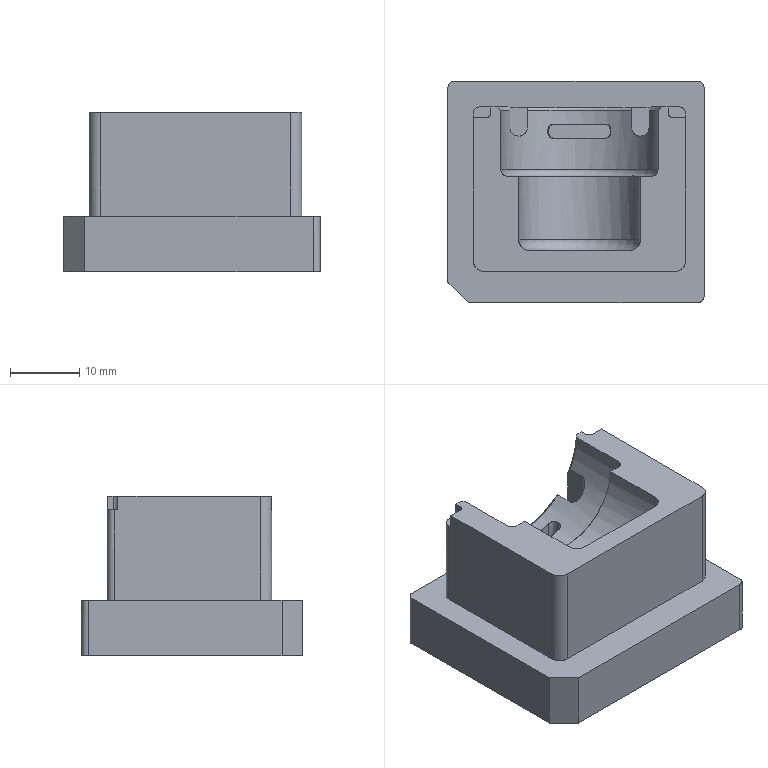NC program | PowerMill | posted with a generic post | part box 37 x 32 x 23 mm
Lines 14663 to 15641 of 253511:
N14760 M6
N14761 S20000 M03
N14762 G00 G90 X0.0 Y0.0
N14763 G43 Z9.8 H26
N14764
N14765 G05 P10000 R4
N14766 X9.0481 Y8.9727
N14767 Z-5.8494
N14768 G01 Z-7.0494 F1800.0
N14769 X9.0521 Y8.9504 F3000.0
N14770 G03 X9.2883 Y8.7865 I0.2001 J0.0361
N14771 G01 X9.4922 Y8.8233
N14772 X9.5753 Y8.871
N14773 X9.5951 Y8.8836
N14774 X9.7263 Y9.0245
N14775 X9.7351 Y9.0362
N14776 X9.7414 Y9.0494
N14777 X9.7735 Y9.1394
N14778 X9.7947 Y9.3383
N14779 X9.796 Y9.5383
N14780 X8.9147 Y8.8373 Z-7.0991
N14781 X8.9212 Y8.8236
N14782 G03 X9.1025 Y8.759 I0.1229 J0.0584
N14783 G01 X9.1066 Y8.761
N14784 X9.4811 Y8.8222
N14785 X9.4936 Y8.8254
N14786 X9.5053 Y8.8308
N14787 X9.5665 Y8.8659
N14788 X9.5964 Y8.8848
N14789 X9.7288 Y9.0272
N14790 X9.738 Y9.0395
N14791 X9.7719 Y9.1349
N14792 X9.7784 Y9.1596
N14793 X9.7953 Y9.3614
N14794 X9.7961 Y9.5638
N14795 X8.8735 Y8.8424 Z-7.1488
N14796 X8.8795 Y8.8285
N14797 G03 X9.0584 Y8.7575 I0.1249 J0.054
N14798 G01 X9.0665 Y8.761
N14799 X9.4821 Y8.8231
N14800 X9.4951 Y8.8263
N14801 X9.5073 Y8.8319
N14802 X9.5578 Y8.8608
N14803 X9.5977 Y8.8861
N14804 X9.7266 Y9.0247
N14805 X9.7384 Y9.0406
N14806 X9.7703 Y9.1303
N14807 X9.7788 Y9.1623
N14808 X9.7957 Y9.3745
N14809 X9.7962 Y9.5873
N14810 X8.8253 Y8.8428 Z-7.1986
N14811 X8.831 Y8.8288
N14812 G03 X9.0082 Y8.7536 I0.1262 J0.051
N14813 G01 X9.0264 Y8.761
N14814 X9.4831 Y8.824
N14815 X9.4965 Y8.8272
N14816 X9.5091 Y8.8328
N14817 X9.5495 Y8.856
N14818 X9.5988 Y8.8873
N14819 X9.7237 Y9.0215
N14820 X9.739 Y9.0421
N14821 X9.7686 Y9.1252
N14822 X9.7791 Y9.1651
N14823 X9.7961 Y9.3878
N14824 X9.7963 Y9.611
N14825 X8.8326 Y8.8948 Z-7.2483
N14826 X8.8345 Y8.8798
N14827 G03 X8.9866 Y8.7618 I0.135 J0.0171
N14828 G01 X9.4868 Y8.8252
N14829 X9.5457 Y8.8529
N14830 X9.6001 Y8.8886
N14831 X9.7211 Y9.0186
N14832 X9.7332 Y9.0349
N14833 X9.7389 Y9.0439
N14834 X9.7432 Y9.0536
N14835 X9.7548 Y9.0864
N14836 X9.7938 Y9.3288
N14837 X9.796 Y9.4402
N14838 X9.7963 Y9.6136
N14839 X8.8159 Y8.8942 Z-7.298
N14840 X8.8178 Y8.8792
N14841 G03 X8.9697 Y8.761 I0.135 J0.0169
N14842 G01 X9.4867 Y8.8257
N14843 X9.5467 Y8.853
N14844 X9.6013 Y8.8899
N14845 X9.7184 Y9.0157
N14846 X9.7337 Y9.0363
N14847 X9.7394 Y9.0453
N14848 X9.7437 Y9.055
N14849 X9.754 Y9.0839
N14850 X9.7939 Y9.3295
N14851 X9.796 Y9.4402
N14852 X9.7964 Y9.6264
N14853 X8.8023 Y8.9071 Z-7.3477
N14854 X8.8034 Y8.892
N14855 G03 X8.949 Y8.7661 I0.1357 J0.0099
N14856 G01 X9.0961 Y8.7768
N14857 X9.4867 Y8.8256
N14858 X9.5047 Y8.8301
N14859 X9.5233 Y8.8408
N14860 X9.6025 Y8.8911
N14861 X9.7158 Y9.0128
N14862 X9.7343 Y9.0377
N14863 X9.7399 Y9.0467
N14864 X9.7442 Y9.0564
N14865 X9.7531 Y9.0814
N14866 X9.7939 Y9.3301
N14867 X9.7961 Y9.4402
N14868 X9.7965 Y9.6404
N14869 X8.7846 Y8.9353 Z-7.3975
N14870 X8.7849 Y8.9202
N14871 G03 X8.924 Y8.787 I0.1361 J0.0029
N14872 G01 X9.2312 Y8.7936
N14873 X9.4868 Y8.8256
N14874 X9.4951 Y8.8277
N14875 X9.5059 Y8.8313
N14876 X9.516 Y8.8367
N14877 X9.6037 Y8.8923
N14878 X9.7133 Y9.01
N14879 X9.7348 Y9.039
N14880 X9.7405 Y9.048
N14881 X9.7448 Y9.0578
N14882 X9.7523 Y9.0788
N14883 X9.794 Y9.3307
N14884 X9.7961 Y9.4402
N14885 X9.7966 Y9.6561
N14886 X8.7278 Y8.9089 Z-7.4472
N14887 X8.7318 Y8.8943
N14888 G03 X8.8989 Y8.7988 I0.1313 J0.0358
N14889 G01 X8.9095 Y8.8016
N14890 X9.2657 Y8.7979
N14891 X9.4845 Y8.8252
N14892 X9.4999 Y8.8289
N14893 X9.5142 Y8.8359
N14894 X9.6048 Y8.8933
N14895 X9.7107 Y9.0072
N14896 X9.7353 Y9.0404
N14897 X9.741 Y9.0494
N14898 X9.7453 Y9.0591
N14899 X9.7514 Y9.0762
N14900 X9.7941 Y9.3313
N14901 X9.7962 Y9.4402
N14902 X9.7967 Y9.6717
N14903 X8.6963 Y8.9063 Z-7.4969
N14904 X8.701 Y8.8919
N14905 G03 X8.8724 Y8.8043 I0.1295 J0.0419
N14906 G01 X8.9095 Y8.8162
N14907 X9.2865 Y8.8004
N14908 X9.4835 Y8.825
N14909 X9.491 Y8.8267
N14910 X9.503 Y8.8305
N14911 X9.5141 Y8.8362
N14912 X9.6058 Y8.8944
N14913 X9.7082 Y9.0044
N14914 X9.7372 Y9.0435
N14915 X9.7433 Y9.0532
N14916 X9.7484 Y9.0676
N14917 X9.7502 Y9.0736
N14918 X9.7515 Y9.0797
N14919 X9.7941 Y9.3319
N14920 X9.7962 Y9.4402
N14921 X9.7967 Y9.687
N14922 X8.6724 Y8.9261 Z-7.5467
N14923 X8.676 Y8.9114
N14924 G03 X8.8411 Y8.8123 I0.1321 J0.033
N14925 G01 X8.9095 Y8.8294
N14926 X9.2996 Y8.802
N14927 X9.4787 Y8.8244
N14928 X9.5034 Y8.8298
N14929 X9.6068 Y8.8954
N14930 X9.7058 Y9.0017
N14931 X9.733 Y9.0357
N14932 X9.7504 Y9.0756
N14933 X9.7942 Y9.3325
N14934 X9.7963 Y9.4402
N14935 X9.7968 Y9.7066
N14936 X8.6362 Y8.9347 Z-7.5964
N14937 X8.6396 Y8.92
N14938 G03 X8.8028 Y8.8178 I0.1327 J0.0304
N14939 G01 X8.9095 Y8.8423
N14940 X9.1037 Y8.8144
N14941 X9.2996 Y8.802
N14942 X9.474 Y8.8238
N14943 X9.5034 Y8.8302
N14944 X9.6079 Y8.8965
N14945 X9.6763 Y8.9664
N14946 X9.7364 Y9.0436
N14947 X9.75 Y9.0755
N14948 X9.7942 Y9.333
N14949 X9.7963 Y9.4402
N14950 X9.7969 Y9.7257
N14951 X8.6211 Y8.9728 Z-7.6461
N14952 X8.6229 Y8.9578
N14953 G03 X8.7743 Y8.8388 I0.1352 J0.0162
N14954 G01 X8.9095 Y8.855
N14955 X9.1215 Y8.8144
N14956 X9.2996 Y8.8019
N14957 X9.4695 Y8.8232
N14958 X9.5034 Y8.8305
N14959 X9.609 Y8.8975
N14960 X9.6767 Y8.967
N14961 X9.7361 Y9.0437
N14962 X9.7496 Y9.0754
N14963 X9.7943 Y9.3335
N14964 X9.7964 Y9.4402
N14965 X9.797 Y9.7457
N14966 X8.5993 Y9.0001 Z-7.6959
N14967 X8.6002 Y8.985
N14968 G03 X8.7438 Y8.8568 I0.1359 J0.0077
N14969 G01 X8.9095 Y8.8663
N14970 X9.1445 Y8.8127
N14971 X9.2996 Y8.8019
N14972 X9.4658 Y8.8226
N14973 X9.5034 Y8.8307
N14974 X9.6098 Y8.8984
N14975 X9.6769 Y8.9674
N14976 X9.7358 Y9.0437
N14977 X9.7493 Y9.0754
N14978 X9.7944 Y9.334
N14979 X9.7964 Y9.4401
N14980 X9.7971 Y9.7667
N14981 X8.5759 Y9.0307 Z-7.7456
N14982 Y9.0156
N14983 G03 X8.7112 Y8.8787 I0.1361 J-0.0008
N14984 G01 X8.9095 Y8.8775
N14985 X9.159 Y8.8117
N14986 X9.2996 Y8.8018
N14987 X9.4621 Y8.8221
N14988 X9.5034 Y8.831
N14989 X9.6106 Y8.8991
N14990 X9.6771 Y8.9679
N14991 X9.7354 Y9.0438
N14992 X9.7489 Y9.0753
N14993 X9.7944 Y9.3345
N14994 X9.7965 Y9.4401
N14995 X9.7972 Y9.7914
N14996 X8.5488 Y9.0652 Z-7.7953
N14997 X8.5477 Y9.0501
N14998 G03 X8.6737 Y8.9045 I0.1357 J-0.0098
N14999 G01 X8.9095 Y8.8875
N15000 X9.1682 Y8.811
N15001 X9.2996 Y8.8018
N15002 X9.4021 Y8.8121
N15003 X9.5034 Y8.8312
N15004 X9.6113 Y8.8999
N15005 X9.6773 Y8.9683
N15006 X9.7351 Y9.0438
N15007 X9.7486 Y9.0752
N15008 X9.7945 Y9.335
N15009 X9.7965 Y9.4401
N15010 X9.7973 Y9.8158
N15011 X8.5378 Y9.1009 Z-7.845
N15012 X8.5358 Y9.0859
N15013 G03 X8.6519 Y8.9324 I0.1348 J-0.0187
N15014 G01 X8.9095 Y8.8967
N15015 X9.1747 Y8.8105
N15016 X9.2996 Y8.8017
N15017 X9.4021 Y8.8123
N15018 X9.5034 Y8.8314
N15019 X9.6122 Y8.9007
N15020 X9.6777 Y8.9688
N15021 X9.7349 Y9.0439
N15022 X9.7483 Y9.0752
N15023 X9.7945 Y9.3355
N15024 X9.7966 Y9.4401
N15025 X9.7974 Y9.8406
N15026 X8.5213 Y9.1399 Z-7.8948
N15027 X8.5183 Y9.1251
N15028 G03 X8.6242 Y8.9643 I0.1333 J-0.0274
N15029 G01 X8.9095 Y8.9058
N15030 X8.9819 Y8.8731
N15031 X9.1663 Y8.8132
N15032 X9.1748 Y8.811
N15033 X9.1835 Y8.8098
N15034 X9.2872 Y8.8025
N15035 X9.3961 Y8.8113
N15036 X9.5034 Y8.8317
N15037 X9.6129 Y8.9014
N15038 X9.6779 Y8.9691
N15039 X9.7346 Y9.0439
N15040 X9.748 Y9.0751
N15041 X9.7946 Y9.3359
N15042 X9.7966 Y9.4401
N15043 X9.7975 Y9.8607
N15044 X8.4398 Y9.1256 Z-7.9445
N15045 X8.4418 Y9.1106
N15046 G03 X8.595 Y8.9941 I0.1349 J0.0183
N15047 G01 X8.6125 Y8.9964
N15048 X8.9095 Y8.9139
N15049 X9.0147 Y8.8624
N15050 X9.1663 Y8.8131
N15051 X9.1748 Y8.8109
N15052 X9.1835 Y8.8098
N15053 X9.2794 Y8.803
N15054 X9.3058 Y8.8024
N15055 X9.4053 Y8.813
N15056 X9.5034 Y8.8319
N15057 X9.6136 Y8.9021
N15058 X9.6781 Y8.9695
N15059 X9.7344 Y9.0439
N15060 X9.7478 Y9.0751
N15061 X9.7947 Y9.3363
N15062 X9.7967 Y9.4401
N15063 X9.7976 Y9.8797
N15064 X8.4182 Y9.1658 Z-7.9942
N15065 X8.4192 Y9.1507
N15066 G03 X8.5644 Y9.0243 I0.1359 J0.0094
N15067 G01 X8.6125 Y9.0276
N15068 X8.9095 Y8.9215
N15069 X9.0341 Y8.856
N15070 X9.1663 Y8.8131
N15071 X9.1748 Y8.8109
N15072 X9.1835 Y8.8097
N15073 X9.3141 Y8.8033
N15074 X9.4439 Y8.8196
N15075 X9.5034 Y8.8321
N15076 X9.6142 Y8.9027
N15077 X9.6783 Y8.9698
N15078 X9.7342 Y9.0439
N15079 X9.7476 Y9.0751
N15080 X9.7947 Y9.3367
N15081 X9.7967 Y9.4401
N15082 X9.7977 Y9.9014
N15083 X8.3834 Y9.2094 Z-8.044
N15084 X8.3835 Y9.1943
N15085 G03 X8.52 Y9.0585 I0.1361 J0.0003
N15086 G01 X8.6125 Y9.0588
N15087 X8.9095 Y8.9268
N15088 X8.9532 Y8.8985
N15089 X9.0341 Y8.856
N15090 X9.1662 Y8.813
N15091 X9.1747 Y8.8108
N15092 X9.1834 Y8.8097
N15093 X9.3445 Y8.8053
N15094 X9.5034 Y8.8323
N15095 X9.6149 Y8.9034
N15096 X9.6785 Y8.9702
N15097 X9.734 Y9.044
N15098 X9.7473 Y9.075
N15099 X9.7948 Y9.3371
N15100 X9.7968 Y9.4401
N15101 X9.7978 Y9.9338
N15102 X8.3624 Y9.2611 Z-8.0937
N15103 X8.3614 Y9.246
N15104 G03 X8.4882 Y9.1012 I0.1358 J-0.009
N15105 G01 X8.6125 Y9.093
N15106 X8.71 Y9.058
N15107 X8.9591 Y8.8953
N15108 X9.034 Y8.8559
N15109 X9.1662 Y8.813
N15110 X9.1747 Y8.8108
N15111 X9.1834 Y8.8096
N15112 X9.3446 Y8.8053
N15113 X9.5034 Y8.8324
N15114 X9.6154 Y8.9038
N15115 X9.6787 Y8.9705
N15116 X9.7337 Y9.044
N15117 X9.747 Y9.075
N15118 X9.7948 Y9.3375
N15119 X9.7968 Y9.4401
N15120 X9.7979 Y9.9604
N15121 X8.3553 Y9.3159 Z-8.1434
N15122 X8.3532 Y9.3009
N15123 G03 X8.4691 Y9.1472 I0.1348 J-0.0189
N15124 G01 X8.6125 Y9.1271
N15125 X8.7552 Y9.058
N15126 X9.0003 Y8.8736
N15127 X9.034 Y8.8559
N15128 X9.1662 Y8.8129
N15129 X9.1747 Y8.8107
N15130 X9.1834 Y8.8096
N15131 X9.2726 Y8.8033
N15132 X9.3027 Y8.8026
N15133 X9.308 Y8.8027
N15134 X9.3133 Y8.8031
N15135 X9.409 Y8.814
N15136 X9.5034 Y8.8326
N15137 X9.6161 Y8.9045
N15138 X9.679 Y8.9708
N15139 X9.7336 Y9.0441
N15140 X9.7468 Y9.0749
N15141 X9.7949 Y9.3379
N15142 X9.7969 Y9.4401
N15143 X9.7981 Y9.9935
N15144 X8.3351 Y9.3805 Z-8.1932
N15145 X8.332 Y9.3657
N15146 G03 X8.4365 Y9.204 I0.1331 J-0.0286
N15147 G01 X8.6125 Y9.1663
N15148 X8.7867 Y9.058
N15149 X8.8761 Y8.967
N15150 X9.0002 Y8.8736
N15151 X9.034 Y8.8558
N15152 X9.167 Y8.8126
N15153 X9.3363 Y8.8047
N15154 X9.5034 Y8.8326
N15155 X9.6166 Y8.9049
N15156 X9.6791 Y8.971
N15157 X9.7334 Y9.0441
N15158 X9.7467 Y9.0749
N15159 X9.7949 Y9.3383
N15160 X9.7969 Y9.4401
N15161 X9.7982 Y10.0278
N15162 X8.3385 Y9.448 Z-8.2429
N15163 X8.3342 Y9.4335
N15164 G03 X8.4259 Y9.2643 I0.1305 J-0.0387
N15165 G01 X8.6125 Y9.2088
N15166 X8.8071 Y9.058
N15167 X8.8916 Y8.9552
N15168 X9.0002 Y8.8735
N15169 X9.034 Y8.8558
N15170 X9.1619 Y8.8142
N15171 X9.3337 Y8.8046
N15172 X9.5034 Y8.8327
N15173 X9.6169 Y8.9052
N15174 X9.6904 Y8.9834
N15175 X9.7466 Y9.0748
N15176 X9.795 Y9.3386
N15177 X9.797 Y9.4401
N15178 X9.7983 Y10.069
N15179 X8.3476 Y9.5238 Z-8.2926
N15180 X8.3421 Y9.5096
N15181 G03 X8.4203 Y9.3337 I0.1271 J-0.0489
N15182 G01 X8.6125 Y9.2597
N15183 X8.8185 Y9.058
N15184 X8.8969 Y8.9512
N15185 X9.0002 Y8.8735
N15186 X9.034 Y8.8557
N15187 X9.1569 Y8.8158
N15188 X9.3311 Y8.8044
N15189 X9.5034 Y8.8327
N15190 X9.6172 Y8.9055
N15191 X9.6904 Y8.9836
N15192 X9.7464 Y9.0748
N15193 X9.7951 Y9.339
N15194 X9.797 Y9.4401
N15195 X9.7985 Y10.1186
N15196 X8.3507 Y9.6176 Z-8.3424
N15197 X8.3441 Y9.604
N15198 G03 X8.4077 Y9.4223 I0.1227 J-0.0591
N15199 G01 X8.6125 Y9.3237
N15200 X8.806 Y9.0701
N15201 X8.8185 Y9.0579
N15202 X8.8905 Y8.9597
N15203 X8.8974 Y8.9517
N15204 X8.9053 Y8.9448
N15205 X9.0002 Y8.8734
N15206 X9.034 Y8.8557
N15207 X9.1516 Y8.8175
N15208 X9.3284 Y8.8042
N15209 X9.5034 Y8.8327
N15210 X9.6175 Y8.9057
N15211 X9.6905 Y8.9837
N15212 X9.7463 Y9.0748
N15213 X9.7951 Y9.3393
N15214 X9.7971 Y9.4401
N15215 X9.7986 Y10.1775
N15216 X8.3896 Y9.7229 Z-8.3921
N15217 X8.3819 Y9.7098
N15218 G03 X8.4298 Y9.5234 I0.1172 J-0.0692
N15219 G01 X8.6125 Y9.4154
N15220 X8.6691 Y9.3549
N15221 X8.8203 Y9.058
N15222 X8.8991 Y8.9494
N15223 X8.9934 Y8.8785
N15224 X9.0036 Y8.8715
N15225 X9.0339 Y8.8556
N15226 X9.1461 Y8.8192
N15227 X9.3256 Y8.804
N15228 X9.5034 Y8.8327
N15229 X9.6177 Y8.9059
N15230 X9.6905 Y8.9838
N15231 X9.7462 Y9.0748
N15232 X9.7952 Y9.3397
N15233 X9.7971 Y9.4401
N15234 X9.7986 Y10.1498
N15235 X9.7987 Y10.2518
N15236 X9.013 Y9.9325 Z-8.4418
N15237 X8.9904
N15238 G03 X8.7874 Y9.729 I0.0003 J-0.2033
N15239 G01 X8.7879 Y9.2015
N15240 X8.8215 Y9.058
N15241 X8.9005 Y8.9483
N15242 X8.9646 Y8.8982
N15243 X9.0339 Y8.8556
N15244 G03 X9.4268 Y8.817 I0.2569 J0.5964
N15245 G01 X9.5034 Y8.8327
N15246 X9.6179 Y8.906
N15247 X9.6905 Y8.9839
N15248 X9.746 Y9.0747
N15249 X9.7952 Y9.34
N15250 X9.7972 Y9.4401
N15251 X9.7986 Y10.1111
N15252 X9.7988 Y10.3366
N15253 X9.0129 Y10.0384 Z-8.4916
N15254 X8.9904
N15255 G03 X8.7873 Y9.835 I0.0002 J-0.2032
N15256 G01 X8.788 Y9.2014
N15257 X8.8221 Y9.058
N15258 X8.9012 Y8.9477
N15259 X8.9768 Y8.8908
N15260 X9.0125 Y8.8668
N15261 X9.0339 Y8.8555
N15262 G03 X9.4261 Y8.8169 I0.2569 J0.5978
N15263 G01 X9.5034 Y8.8327
N15264 X9.6181 Y8.9061
N15265 X9.6905 Y8.9839
N15266 X9.7459 Y9.0747
N15267 X9.7953 Y9.3404
N15268 X9.7972 Y9.4401
N15269 X9.7986 Y10.0728
N15270 X9.7989 Y10.4432
N15271 X8.3717 Y12.6667 Z-8.5413
N15272 X8.363 Y12.6544
N15273 G03 X8.3959 Y12.4647 I0.1113 J-0.0784
N15274 G01 X8.5946 Y12.3248
N15275 X8.7572 Y12.0278
N15276 X8.7854 Y11.7308
N15277 X8.788 Y9.2013
N15278 X8.823 Y9.058
N15279 X8.9022 Y8.9469
N15280 X8.9687 Y8.8969
N15281 X9.0171 Y8.8643
N15282 G03 X9.4254 Y8.8167 I0.2743 J0.5782
N15283 G01 X9.5034 Y8.8327
N15284 X9.6184 Y8.9064
N15285 X9.6906 Y8.9841
N15286 X9.7458 Y9.0746
N15287 X9.7953 Y9.3407
N15288 X9.7973 Y9.4401
N15289 X9.7985 Y10.0346
N15290 X9.8004 Y12.3153
N15291 X9.894 Y12.6217
N15292 X10.0096 Y12.7538
N15293 X8.3678 Y12.7082 Z-8.591
N15294 X8.3589 Y12.696
N15295 G03 X8.3886 Y12.5058 I0.1099 J-0.0802
N15296 G01 X8.6125 Y12.3425
N15297 X8.7669 Y12.0278
N15298 X8.7854 Y11.7308
N15299 X8.7882 Y9.2012
N15300 X8.8196 Y9.0754
N15301 X8.8357 Y9.0444
N15302 X8.9545 Y8.9075
N15303 X8.9687 Y8.8968
N15304 X8.9954 Y8.8788
N15305 X9.1992 Y8.808
N15306 X9.3524 Y8.8065
N15307 X9.5034 Y8.8327
N15308 X9.6186 Y8.9065
N15309 X9.6907 Y8.9841
N15310 X9.7458 Y9.0746
N15311 X9.7954 Y9.341
N15312 X9.7973 Y9.4401
N15313 X9.7985 Y9.9963
N15314 X9.8004 Y12.3153
N15315 X9.894 Y12.6217
N15316 X10.0212 Y12.7671
N15317 X8.3645 Y12.7485 Z-8.6407
N15318 X8.3556 Y12.7362
N15319 G03 X8.3853 Y12.546 I0.1099 J-0.0802
N15320 G01 X8.6125 Y12.3803
N15321 X8.7736 Y12.0278
N15322 X8.7752 Y11.8791
N15323 X8.7853 Y11.7308
N15324 X8.7881 Y9.2615
N15325 X8.7884 Y9.2011
N15326 X8.8204 Y9.0751
N15327 X8.8364 Y9.0445
N15328 X8.9561 Y8.9062
N15329 X8.9686 Y8.8968
N15330 X8.9938 Y8.8799
N15331 X9.1999 Y8.8079
N15332 X9.3528 Y8.8065
N15333 X9.5034 Y8.8327
N15334 X9.6187 Y8.9066
N15335 X9.6907 Y8.9842
N15336 X9.7457 Y9.0746
N15337 X9.7954 Y9.3413
N15338 X9.7974 Y9.4401
N15339 X9.7985 Y9.958
N15340 X9.8004 Y12.3153
N15341 X9.894 Y12.6217
N15342 X10.035 Y12.7829
N15343 X8.384 Y12.772 Z-8.6905
N15344 X8.3751 Y12.7598
N15345 G03 X8.4048 Y12.5696 I0.1099 J-0.0802
N15346 G01 X8.6125 Y12.4181
N15347 X8.6781 Y12.3248
N15348 X8.7801 Y12.0278
N15349 X8.789 Y10.6144
N15350 X8.7886 Y9.2011
N15351 X8.8241 Y9.0642
N15352 X8.8364 Y9.0445
N15353 X8.954 Y8.9086
N15354 X9.0003 Y8.8775
N15355 X9.1908 Y8.811
N15356 X9.2 Y8.8085
N15357 X9.2095 Y8.8072
N15358 X9.3576 Y8.8069
N15359 X9.5034 Y8.8327
N15360 X9.619 Y8.9067
N15361 X9.6908 Y8.9843
N15362 X9.7457 Y9.0746
N15363 X9.7955 Y9.3416
N15364 X9.7974 Y9.4401
N15365 X9.7984 Y9.9196
N15366 X9.8004 Y12.3153
N15367 X9.894 Y12.6217
N15368 X10.0471 Y12.7967
N15369 X8.4277 Y12.8178 Z-8.7402
N15370 X8.4178 Y12.8063
N15371 G03 X8.4326 Y12.6143 I0.1034 J-0.0886
N15372 G01 X8.6125 Y12.4603
N15373 X8.7005 Y12.3248
N15374 X8.7834 Y12.0278
N15375 X8.7836 Y11.7569
N15376 X8.7852 Y11.7308
N15377 X8.7878 Y9.4661
N15378 X8.7885 Y9.2148
N15379 X8.7888 Y9.201
N15380 X8.8233 Y9.0707
N15381 X8.8293 Y9.0555
N15382 X8.8385 Y9.042
N15383 X8.9519 Y8.9109
N15384 X9.0026 Y8.8767
N15385 X9.1908 Y8.811
N15386 X9.2 Y8.8084
N15387 X9.2094 Y8.8071
N15388 X9.3576 Y8.8069
N15389 X9.5034 Y8.8327
N15390 X9.6191 Y8.9069
N15391 X9.6909 Y8.9844
N15392 X9.7457 Y9.0746
N15393 X9.7956 Y9.3419
N15394 X9.7975 Y9.4401
N15395 X9.7984 Y9.8807
N15396 X9.8004 Y12.3153
N15397 X9.894 Y12.6217
N15398 X10.0589 Y12.8102
N15399 X8.3826 Y12.8462 Z-8.7899
N15400 X8.3752 Y12.833
N15401 G03 X8.4279 Y12.6478 I0.1189 J-0.0663
N15402 G01 X8.4748 Y12.6217
N15403 X8.6125 Y12.4937
N15404 X8.7171 Y12.3248
N15405 X8.7853 Y12.0278
N15406 Y11.6291
N15407 X8.7877 Y9.4661
N15408 X8.7885 Y9.2249
N15409 X8.789 Y9.2009
N15410 X8.8275 Y9.058
N15411 X8.8395 Y9.0407
N15412 X8.9503 Y8.9126
N15413 X9.0043 Y8.876
N15414 X9.1907 Y8.8109
N15415 X9.1999 Y8.8084
N15416 X9.2094 Y8.8071
N15417 X9.3576 Y8.8068
N15418 X9.5034 Y8.8327
N15419 X9.6193 Y8.907
N15420 X9.691 Y8.9844
N15421 X9.7457 Y9.0746
N15422 X9.7956 Y9.3422
N15423 X9.7975 Y9.4401
N15424 X9.7984 Y9.8424
N15425 X9.8004 Y12.3153
N15426 X9.894 Y12.6217
N15427 X10.0634 Y12.8153
N15428 X8.3951 Y12.8768 Z-8.8397
N15429 X8.3873 Y12.8639
N15430 G03 X8.4328 Y12.6768 I0.1163 J-0.0708
N15431 G01 X8.5233 Y12.6217
N15432 X8.6125 Y12.5315
N15433 X8.7333 Y12.3248
N15434 X8.7854 Y12.0278
N15435 Y11.4772
N15436 X8.7877 Y9.4661
N15437 X8.7884 Y9.2347
N15438 X8.7892 Y9.2008
N15439 X8.8284 Y9.058
N15440 X8.8442 Y9.0353
N15441 X8.9485 Y8.9147
N15442 X9.0062 Y8.8753
N15443 X9.1907 Y8.8109
N15444 X9.1999 Y8.8084
N15445 X9.2094 Y8.807
N15446 X9.3575 Y8.8068
N15447 X9.5034 Y8.8327
N15448 X9.6195 Y8.9071
N15449 X9.691 Y8.9845
N15450 X9.7457 Y9.0746
N15451 X9.7957 Y9.3425
N15452 X9.7976 Y9.4401
N15453 X9.7983 Y9.804
N15454 X9.8004 Y12.3153
N15455 X9.894 Y12.6217
N15456 X10.0677 Y12.8202
N15457 X8.4147 Y12.9018 Z-8.8894
N15458 X8.4063 Y12.8892
N15459 G03 X8.4448 Y12.7005 I0.1136 J-0.0751
N15460 G01 X8.564 Y12.6217
N15461 X8.7468 Y12.3248
N15462 X8.7854 Y12.0278
N15463 Y11.4313
N15464 X8.7876 Y9.4661
N15465 X8.7883 Y9.2435
N15466 X8.7894 Y9.2007
N15467 X8.8293 Y9.058
N15468 X8.8487 Y9.0299
N15469 X8.9466 Y8.9168
N15470 X9.0079 Y8.8747
N15471 X9.1907 Y8.8108
N15472 X9.1999 Y8.8083
N15473 X9.2094 Y8.807
N15474 X9.3575 Y8.8068
N15475 X9.5034 Y8.8327
N15476 X9.6196 Y8.9072
N15477 X9.6911 Y8.9846
N15478 X9.7457 Y9.0746
N15479 X9.7957 Y9.3429
N15480 X9.7976 Y9.4401
N15481 X9.7983 Y9.7656
N15482 X9.8004 Y12.3153
N15483 X9.894 Y12.6217
N15484 X10.0721 Y12.8253
N15485 X8.4336 Y12.9253 Z-8.9391
N15486 X8.4249 Y12.913
N15487 G03 X8.4565 Y12.7231 I0.1107 J-0.0791
N15488 G01 X8.5985 Y12.6217
N15489 X8.7585 Y12.3248
N15490 X8.7854 Y12.0278
N15491 X8.7851 Y10.6096
N15492 X8.792 Y9.1914
N15493 X8.828 Y9.0622
N15494 X8.8823 Y8.9872
N15495 X8.9448 Y8.9188
N15496 X9.0095 Y8.8741
N15497 X9.1907 Y8.8108
N15498 X9.1999 Y8.8083
N15499 X9.2094 Y8.807
N15500 X9.3575 Y8.8068
N15501 X9.5034 Y8.8327
N15502 X9.6198 Y8.9073
N15503 X9.6912 Y8.9846
N15504 X9.7457 Y9.0746
N15505 X9.7958 Y9.3432
N15506 X9.7977 Y9.4401
N15507 X9.7983 Y9.7271
N15508 X9.8004 Y12.3153
N15509 X9.894 Y12.6217
N15510 X10.0745 Y12.828
N15511 X8.4543 Y12.9476 Z-8.9889
N15512 X8.4454 Y12.9354
N15513 G03 X8.4751 Y12.7452 I0.1099 J-0.0802
N15514 G01 X8.6125 Y12.645
N15515 X8.7671 Y12.3248
N15516 X8.7854 Y12.0278
N15517 Y11.3398
N15518 X8.7875 Y9.4661
N15519 X8.7879 Y9.3351
N15520 X8.8186 Y9.0958
N15521 X8.8244 Y9.075
N15522 X8.8285 Y9.0639
N15523 X8.8344 Y9.0537
N15524 X8.8586 Y9.0183
N15525 X8.943 Y8.9208
N15526 X9.0109 Y8.8735
N15527 X9.1907 Y8.8107
N15528 X9.1999 Y8.8082
N15529 X9.2094 Y8.8069
N15530 X9.3575 Y8.8067
N15531 X9.5034 Y8.8327
N15532 X9.62 Y8.9074
N15533 X9.6913 Y8.9847
N15534 X9.7457 Y9.0746
N15535 X9.7958 Y9.3435
N15536 X9.7977 Y9.4401
N15537 X9.7983 Y9.6887
N15538 X9.8004 Y12.3153
N15539 X9.894 Y12.6217
N15540 X10.0764 Y12.8301
N15541 X8.4513 Y12.973 Z-9.0386
N15542 X8.4429 Y12.9605
N15543 G03 X8.4801 Y12.7716 I0.113 J-0.0759
N15544 G01 X8.6125 Y12.6828
N15545 X8.6572 Y12.6217
N15546 X8.7755 Y12.3248
N15547 X8.7854 Y12.0278
N15548 Y11.2942
N15549 X8.7875 Y9.4661
N15550 X8.7879 Y9.3355
N15551 X8.8186 Y9.0956
N15552 X8.8237 Y9.0775
N15553 X8.8277 Y9.0665
N15554 X8.8335 Y9.0563
N15555 X8.8836 Y8.9864
N15556 X8.9413 Y8.9227
N15557 X9.0122 Y8.873
N15558 X9.1907 Y8.8107
N15559 X9.1999 Y8.8082
N15560 X9.2093 Y8.8069
N15561 X9.3575 Y8.8067
N15562 X9.5034 Y8.8327
N15563 X9.6202 Y8.9075
N15564 X9.6913 Y8.9848
N15565 X9.7457 Y9.0746
N15566 X9.7959 Y9.3438
N15567 X9.7978 Y9.4401
N15568 X9.7982 Y9.6502
N15569 X9.8004 Y12.3153
N15570 X9.894 Y12.6217
N15571 X10.0789 Y12.833
N15572 X8.4699 Y13.0118 Z-9.0883
N15573 X8.461 Y12.9996
N15574 G03 X8.4907 Y12.8094 I0.1099 J-0.0802
N15575 G01 X8.6125 Y12.7206
N15576 X8.6816 Y12.6217
N15577 X8.7805 Y12.3248
N15578 X8.7872 Y10.8303
N15579 X8.7878 Y9.3359
N15580 X8.8186 Y9.0954
N15581 X8.8232 Y9.0789
N15582 X8.8273 Y9.0679
N15583 X8.8331 Y9.0577
N15584 X8.8825 Y8.9881
N15585 X8.9396 Y8.9246
N15586 X9.0133 Y8.8726
N15587 X9.1907 Y8.8106
N15588 X9.1999 Y8.8081
N15589 X9.2093 Y8.8068
N15590 X9.3575 Y8.8067
N15591 X9.5034 Y8.8327
N15592 X9.6203 Y8.9076
N15593 X9.6914 Y8.9848
N15594 X9.7457 Y9.0746
N15595 X9.7959 Y9.3441
N15596 X9.7978 Y9.4401
N15597 X9.7982 Y9.6118
N15598 X9.8004 Y12.3153
N15599 X9.894 Y12.6217
N15600 X10.0872 Y12.8425
N15601 X8.4554 Y13.0353 Z-9.1381
N15602 X8.4465 Y13.0231
N15603 G03 X8.4762 Y12.8329 I0.1099 J-0.0802
N15604 G01 X8.6125 Y12.7335
N15605 X8.6894 Y12.6217
N15606 X8.782 Y12.3248
N15607 X8.7854 Y12.0278
N15608 Y11.2027
N15609 X8.7874 Y9.4661
N15610 X8.7878 Y9.3359
N15611 X8.8153 Y9.1209
N15612 X8.8332 Y9.0592
N15613 X8.8692 Y9.0059
N15614 X8.938 Y8.9264
N15615 X9.0143 Y8.8722
N15616 X9.1907 Y8.8106
N15617 X9.1999 Y8.8081
N15618 X9.2093 Y8.8068
N15619 X9.3575 Y8.8066
N15620 X9.5034 Y8.8327
N15621 X9.6205 Y8.9077
N15622 X9.6915 Y8.9849
N15623 X9.7457 Y9.0746
N15624 X9.796 Y9.3444
N15625 X9.7979 Y9.4401
N15626 X9.7982 Y9.5726
N15627 X9.8004 Y12.3153
N15628 X9.894 Y12.6217
N15629 X10.0955 Y12.8519
N15630 X8.4322 Y13.0522 Z-9.1878
N15631 X8.4233 Y13.04
N15632 G03 X8.453 Y12.8498 I0.11 J-0.0802
N15633 G01 X8.6125 Y12.7335
N15634 X8.6894 Y12.6217
N15635 X8.782 Y12.3248
N15636 X8.7854 Y12.0278
N15637 Y11.1573
N15638 X8.7873 Y9.4661
N15639 X8.7877 Y9.3359
N15640 X8.8145 Y9.1266
N15641 X8.8339 Y9.0596
N15642 X8.8727 Y9.0017
N15643 X8.9362 Y8.9283
N15644 X9.0152 Y8.8718
N15645 X9.1906 Y8.8106
N15646 X9.1998 Y8.808
N15647 X9.2093 Y8.8067
N15648 X9.3575 Y8.8066
N15649 X9.5034 Y8.8327
N15650 X9.6207 Y8.9078
N15651 X9.6915 Y8.985
N15652 X9.7457 Y9.0746
N15653 X9.7961 Y9.3447
N15654 X9.7979 Y9.4401
N15655 X9.7981 Y9.5341
N15656 X9.8004 Y12.3153
N15657 X9.894 Y12.6217
N15658 X10.0955 Y12.8519
N15659 X8.4322 Y13.0522 Z-9.2375
N15660 X8.4233 Y13.04
N15661 G03 X8.453 Y12.8498 I0.11 J-0.0802
N15662 G01 X8.6125 Y12.7335
N15663 X8.6894 Y12.6217
N15664 X8.782 Y12.3248
N15665 X8.7854 Y12.0278
N15666 Y11.1116
N15667 X8.7873 Y9.4661
N15668 X8.7877 Y9.3358
N15669 X8.8138 Y9.1322
N15670 X8.8356 Y9.058
N15671 X8.9131 Y8.9525
N15672 X9.0159 Y8.8715
N15673 X9.1906 Y8.8105
N15674 X9.1998 Y8.808
N15675 X9.2093 Y8.8067
N15676 X9.3575 Y8.8066
N15677 X9.5034 Y8.8327
N15678 X9.6208 Y8.9079
N15679 X9.6916 Y8.985
N15680 X9.7457 Y9.0746
N15681 X9.7961 Y9.345
N15682 X9.798 Y9.4401
N15683 X9.7981 Y9.4955
N15684 X9.8004 Y12.3153
N15685 X9.894 Y12.6217
N15686 X10.0955 Y12.8519
N15687 X8.4322 Y13.0522 Z-9.2872
N15688 X8.4233 Y13.04
N15689 G03 X8.453 Y12.8498 I0.11 J-0.0802
N15690 G01 X8.6125 Y12.7335
N15691 X8.6894 Y12.6217
N15692 X8.782 Y12.3248
N15693 X8.7854 Y12.0278
N15694 Y11.0668
N15695 X8.7872 Y9.4661
N15696 X8.7876 Y9.3358
N15697 X8.8131 Y9.1372
N15698 X8.8363 Y9.058
N15699 X8.9136 Y8.9522
N15700 X9.0165 Y8.8712
N15701 X9.1929 Y8.8097
N15702 X9.3493 Y8.8057
N15703 X9.5034 Y8.8327
N15704 X9.621 Y8.9081
N15705 X9.6917 Y8.9851
N15706 X9.7457 Y9.0746
N15707 X9.7962 Y9.3453
N15708 X9.798 Y9.4401
N15709 X9.7981 Y9.457
N15710 X9.8004 Y12.3153
N15711 X9.894 Y12.6217
N15712 X10.0955 Y12.8519
N15713 X8.4322 Y13.0522 Z-9.337
N15714 X8.4233 Y13.04
N15715 G03 X8.453 Y12.8498 I0.11 J-0.0802
N15716 G01 X8.6125 Y12.7335
N15717 X8.6894 Y12.6217
N15718 X8.782 Y12.3248
N15719 X8.7854 Y12.0278
N15720 Y11.0212
N15721 X8.7872 Y9.4661
N15722 X8.7876 Y9.3358
N15723 X8.8124 Y9.1423
N15724 X8.8369 Y9.058
N15725 X8.914 Y8.952
N15726 X9.017 Y8.871
N15727 X9.192 Y8.8099
N15728 X9.3488 Y8.8056
N15729 X9.5034 Y8.8327
N15730 X9.6212 Y8.9082
N15731 X9.6918 Y8.9852
N15732 X9.7457 Y9.0746
N15733 X9.7962 Y9.3456
N15734 X9.798 Y9.4386
N15735 X9.8004 Y12.3153
N15736 X9.894 Y12.6217
N15737 X10.0955 Y12.8519
N15738 X8.4322 Y13.0522 Z-9.3867